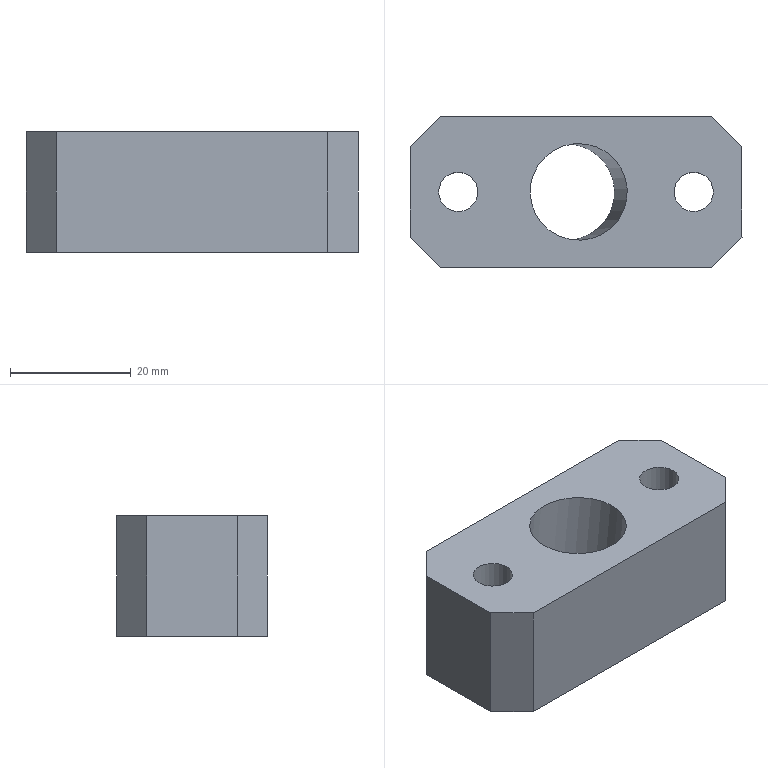Part | STEP file | P011002L001-002 | 1 solid | 17 faces | box 55 x 25 x 20 mm | volume 20325 mm3 | plane 12 | cylinder 5 | commonest cylinder face diameters 6.5 x2 11 x2 16 x1
STEP:
#1=CARTESIAN_POINT('',(0.,0.,0.));
#2=DIRECTION('',(0.,0.,1.));
#3=DIRECTION('',(1.,0.,0.));
#4=AXIS2_PLACEMENT_3D('',#1,#2,#3);
#5=CARTESIAN_POINT('',(-31.537,68.96,-131.));
#6=VERTEX_POINT('',#5);
#7=CARTESIAN_POINT('',(-34.787,68.96,-131.));
#8=DIRECTION('',(0.,0.,-1.));
#9=DIRECTION('',(1.,0.,0.));
#10=AXIS2_PLACEMENT_3D('',#7,#8,#9);
#11=CIRCLE('',#10,3.25);
#12=CARTESIAN_POINT('',(-76.791,76.46,-131.));
#13=DIRECTION('',(0.,0.,-1.));
#14=DIRECTION('',(-1.,0.,0.));
#15=AXIS2_PLACEMENT_3D('',#12,#13,#14);
#16=PLANE('',#15);
#17=CARTESIAN_POINT('',(-42.004,-7.5));
#18=DIRECTION('',(-1.,0.));
#19=AXIS2_PLACEMENT_2D('',#17,#18);
#20=CIRCLE('',#19,3.25);
#21=(GEOMETRIC_REPRESENTATION_CONTEXT(2)PARAMETRIC_REPRESENTATION_CONTEXT()REPRESENTATION_CONTEXT('',''));
#22=DEFINITIONAL_REPRESENTATION('',(#20),#21);
#23=PCURVE('',#16,#22);
#24=CARTESIAN_POINT('',(-34.787,68.96,-113.));
#25=DIRECTION('',(0.,0.,-1.));
#26=DIRECTION('',(1.,0.,0.));
#27=AXIS2_PLACEMENT_3D('',#24,#25,#26);
#28=CYLINDRICAL_SURFACE('',#27,3.25);
#29=CARTESIAN_POINT('',(0.,18.));
#30=DIRECTION('',(1.,0.));
#31=VECTOR('',#30,1.);
#32=LINE('',#29,#31);
#33=(GEOMETRIC_REPRESENTATION_CONTEXT(2)PARAMETRIC_REPRESENTATION_CONTEXT()REPRESENTATION_CONTEXT('',''));
#34=DEFINITIONAL_REPRESENTATION('',(#32),#33);
#35=PCURVE('',#28,#34);
#36=SURFACE_CURVE('',#11,(#23,#35),.PCURVE_S1.);
#37=EDGE_CURVE('',#6,#6,#36,.T.);
#38=ORIENTED_EDGE('',*,*,#37,.T.);
#39=EDGE_LOOP('',(#38));
#40=FACE_BOUND('',#39,.T.);
#41=CARTESIAN_POINT('',(-61.873,68.96,-131.));
#42=VERTEX_POINT('',#41);
#43=CARTESIAN_POINT('',(-53.828,68.96,-131.));
#44=DIRECTION('',(0.,0.,1.));
#45=DIRECTION('',(-1.,0.000000906,0.));
#46=AXIS2_PLACEMENT_3D('',#43,#44,#45);
#47=ELLIPSE('',#46,8.044,8.);
#48=CARTESIAN_POINT('',(-14.919,-7.5));
#49=CARTESIAN_POINT('',(-14.919,-21.356));
#50=CARTESIAN_POINT('',(-26.985,-14.428));
#51=CARTESIAN_POINT('',(-39.051,-7.5));
#52=CARTESIAN_POINT('',(-26.985,-0.5718));
#53=CARTESIAN_POINT('',(-14.919,6.356));
#54=CARTESIAN_POINT('',(-14.919,-7.5));
#55=(BOUNDED_CURVE()B_SPLINE_CURVE(2,(#48,#49,#50,#51,#52,#53,#54),.UNSPECIFIED.,.T.,.F.)B_SPLINE_CURVE_WITH_KNOTS((1,2,2,2,2,1),(-2.094,0.,2.094,4.189,6.283,8.378),.UNSPECIFIED.)CURVE()GEOMETRIC_REPRESENTATION_ITEM()RATIONAL_B_SPLINE_CURVE((1.,0.5,1.,0.5,1.,0.5,1.))REPRESENTATION_ITEM(''));
#56=(GEOMETRIC_REPRESENTATION_CONTEXT(2)PARAMETRIC_REPRESENTATION_CONTEXT()REPRESENTATION_CONTEXT('',''));
#57=DEFINITIONAL_REPRESENTATION('',(#55),#56);
#58=PCURVE('',#16,#57);
#59=CARTESIAN_POINT('',(-49.389,68.96,-88.759));
#60=DIRECTION('',(-0.1045,0.000000095,-0.9945));
#61=DIRECTION('',(0.9945,0.,-0.1045));
#62=AXIS2_PLACEMENT_3D('',#59,#60,#61);
#63=CYLINDRICAL_SURFACE('',#62,8.);
#64=CARTESIAN_POINT('',(9.425,43.315));
#65=CARTESIAN_POINT('',(9.33,43.315));
#66=CARTESIAN_POINT('',(9.139,43.292));
#67=CARTESIAN_POINT('',(8.854,43.191));
#68=CARTESIAN_POINT('',(8.568,43.032));
#69=CARTESIAN_POINT('',(8.282,42.828));
#70=CARTESIAN_POINT('',(7.997,42.595));
#71=CARTESIAN_POINT('',(7.711,42.353));
#72=CARTESIAN_POINT('',(7.426,42.12));
#73=CARTESIAN_POINT('',(7.14,41.916));
#74=CARTESIAN_POINT('',(6.854,41.757));
#75=CARTESIAN_POINT('',(6.569,41.656));
#76=CARTESIAN_POINT('',(6.283,41.622));
#77=CARTESIAN_POINT('',(5.998,41.656));
#78=CARTESIAN_POINT('',(5.712,41.757));
#79=CARTESIAN_POINT('',(5.426,41.916));
#80=CARTESIAN_POINT('',(5.141,42.12));
#81=CARTESIAN_POINT('',(4.855,42.353));
#82=CARTESIAN_POINT('',(4.57,42.595));
#83=CARTESIAN_POINT('',(4.284,42.828));
#84=CARTESIAN_POINT('',(3.998,43.032));
#85=CARTESIAN_POINT('',(3.713,43.191));
#86=CARTESIAN_POINT('',(3.427,43.292));
#87=CARTESIAN_POINT('',(3.237,43.315));
#88=CARTESIAN_POINT('',(3.142,43.315));
#89=B_SPLINE_CURVE_WITH_KNOTS('',3,(#64,#65,#66,#67,#68,#69,#70,#71,#72,#73,#74,#75,#76,#77,#78,#79,#80,#81,#82,#83,#84,#85,#86,#87,#88),.UNSPECIFIED.,.F.,.F.,(4,1,1,1,1,1,1,1,1,1,1,1,1,1,1,1,1,1,1,1,1,1,4),(0.,0.2856,0.5712,0.8568,1.142,1.428,1.714,1.999,2.285,2.57,2.856,3.142,3.427,3.713,3.998,4.284,4.57,4.855,5.141,5.426,5.712,5.998,6.283),.QUASI_UNIFORM_KNOTS.);
#90=(GEOMETRIC_REPRESENTATION_CONTEXT(2)PARAMETRIC_REPRESENTATION_CONTEXT()REPRESENTATION_CONTEXT('',''));
#91=DEFINITIONAL_REPRESENTATION('',(#89),#90);
#92=PCURVE('',#63,#91);
#93=SURFACE_CURVE('',#47,(#58,#92),.PCURVE_S1.);
#94=EDGE_CURVE('',#42,#42,#93,.T.);
#95=ORIENTED_EDGE('',*,*,#94,.F.);
#96=EDGE_LOOP('',(#95));
#97=FACE_BOUND('',#96,.T.);
#98=CARTESIAN_POINT('',(-76.787,81.46,-131.));
#99=VERTEX_POINT('',#98);
#100=CARTESIAN_POINT('',(-31.787,81.46,-131.));
#101=VERTEX_POINT('',#100);
#102=CARTESIAN_POINT('',(-76.791,81.46,-131.));
#103=DIRECTION('',(1.,0.,0.));
#104=VECTOR('',#103,1.);
#105=LINE('',#102,#104);
#106=CARTESIAN_POINT('',(0.,5.));
#107=DIRECTION('',(-1.,0.));
#108=VECTOR('',#107,1.);
#109=LINE('',#106,#108);
#110=(GEOMETRIC_REPRESENTATION_CONTEXT(2)PARAMETRIC_REPRESENTATION_CONTEXT()REPRESENTATION_CONTEXT('',''));
#111=DEFINITIONAL_REPRESENTATION('',(#109),#110);
#112=PCURVE('',#16,#111);
#113=CARTESIAN_POINT('',(-179.787,81.46,-246.));
#114=DIRECTION('',(0.,-1.,0.));
#115=DIRECTION('',(1.,0.,0.));
#116=AXIS2_PLACEMENT_3D('',#113,#114,#115);
#117=PLANE('',#116);
#118=CARTESIAN_POINT('',(102.996,115.));
#119=DIRECTION('',(1.,0.));
#120=VECTOR('',#119,1.);
#121=LINE('',#118,#120);
#122=(GEOMETRIC_REPRESENTATION_CONTEXT(2)PARAMETRIC_REPRESENTATION_CONTEXT()REPRESENTATION_CONTEXT('',''));
#123=DEFINITIONAL_REPRESENTATION('',(#121),#122);
#124=PCURVE('',#117,#123);
#125=SURFACE_CURVE('',#105,(#112,#124),.PCURVE_S1.);
#126=EDGE_CURVE('',#99,#101,#125,.T.);
#127=ORIENTED_EDGE('',*,*,#126,.F.);
#128=CARTESIAN_POINT('',(-81.787,76.46,-131.));
#129=VERTEX_POINT('',#128);
#130=CARTESIAN_POINT('',(-81.787,76.46,-131.));
#131=DIRECTION('',(-0.7071,-0.7071,0.));
#132=VECTOR('',#131,1.);
#133=LINE('',#130,#132);
#134=CARTESIAN_POINT('',(4.996,-0.00000231));
#135=DIRECTION('',(0.7071,-0.7071));
#136=VECTOR('',#135,1.);
#137=LINE('',#134,#136);
#138=(GEOMETRIC_REPRESENTATION_CONTEXT(2)PARAMETRIC_REPRESENTATION_CONTEXT()REPRESENTATION_CONTEXT('',''));
#139=DEFINITIONAL_REPRESENTATION('',(#137),#138);
#140=PCURVE('',#16,#139);
#141=CARTESIAN_POINT('',(-81.787,76.46,-246.));
#142=DIRECTION('',(0.7071,-0.7071,0.));
#143=DIRECTION('',(0.7071,0.7071,0.));
#144=AXIS2_PLACEMENT_3D('',#141,#142,#143);
#145=PLANE('',#144);
#146=CARTESIAN_POINT('',(0.,115.));
#147=DIRECTION('',(-1.,0.));
#148=VECTOR('',#147,1.);
#149=LINE('',#146,#148);
#150=(GEOMETRIC_REPRESENTATION_CONTEXT(2)PARAMETRIC_REPRESENTATION_CONTEXT()REPRESENTATION_CONTEXT('',''));
#151=DEFINITIONAL_REPRESENTATION('',(#149),#150);
#152=PCURVE('',#145,#151);
#153=SURFACE_CURVE('',#133,(#140,#152),.PCURVE_S1.);
#154=EDGE_CURVE('',#99,#129,#153,.T.);
#155=ORIENTED_EDGE('',*,*,#154,.T.);
#156=CARTESIAN_POINT('',(-81.787,61.46,-131.));
#157=VERTEX_POINT('',#156);
#158=CARTESIAN_POINT('',(-81.787,76.46,-131.));
#159=DIRECTION('',(0.,1.,0.));
#160=VECTOR('',#159,1.);
#161=LINE('',#158,#160);
#162=CARTESIAN_POINT('',(4.996,0.));
#163=DIRECTION('',(0.,1.));
#164=VECTOR('',#163,1.);
#165=LINE('',#162,#164);
#166=(GEOMETRIC_REPRESENTATION_CONTEXT(2)PARAMETRIC_REPRESENTATION_CONTEXT()REPRESENTATION_CONTEXT('',''));
#167=DEFINITIONAL_REPRESENTATION('',(#165),#166);
#168=PCURVE('',#16,#167);
#169=CARTESIAN_POINT('',(-81.787,-9.04,-246.));
#170=DIRECTION('',(1.,0.,0.));
#171=DIRECTION('',(0.,0.,1.));
#172=AXIS2_PLACEMENT_3D('',#169,#170,#171);
#173=PLANE('',#172);
#174=CARTESIAN_POINT('',(115.,-85.5));
#175=DIRECTION('',(0.,-1.));
#176=VECTOR('',#175,1.);
#177=LINE('',#174,#176);
#178=(GEOMETRIC_REPRESENTATION_CONTEXT(2)PARAMETRIC_REPRESENTATION_CONTEXT()REPRESENTATION_CONTEXT('',''));
#179=DEFINITIONAL_REPRESENTATION('',(#177),#178);
#180=PCURVE('',#173,#179);
#181=SURFACE_CURVE('',#161,(#168,#180),.PCURVE_S1.);
#182=EDGE_CURVE('',#157,#129,#181,.T.);
#183=ORIENTED_EDGE('',*,*,#182,.F.);
#184=CARTESIAN_POINT('',(-76.787,56.46,-131.));
#185=VERTEX_POINT('',#184);
#186=CARTESIAN_POINT('',(-76.787,56.46,-131.));
#187=DIRECTION('',(0.7071,-0.7071,0.));
#188=VECTOR('',#187,1.);
#189=LINE('',#186,#188);
#190=CARTESIAN_POINT('',(-0.004358,-20.));
#191=DIRECTION('',(-0.7071,-0.7071));
#192=VECTOR('',#191,1.);
#193=LINE('',#190,#192);
#194=(GEOMETRIC_REPRESENTATION_CONTEXT(2)PARAMETRIC_REPRESENTATION_CONTEXT()REPRESENTATION_CONTEXT('',''));
#195=DEFINITIONAL_REPRESENTATION('',(#193),#194);
#196=PCURVE('',#16,#195);
#197=CARTESIAN_POINT('',(-76.787,56.46,-131.));
#198=DIRECTION('',(-0.7071,-0.7071,0.));
#199=DIRECTION('',(0.7071,-0.7071,0.));
#200=AXIS2_PLACEMENT_3D('',#197,#198,#199);
#201=PLANE('',#200);
#202=CARTESIAN_POINT('',(0.,0.));
#203=DIRECTION('',(1.,0.));
#204=VECTOR('',#203,1.);
#205=LINE('',#202,#204);
#206=(GEOMETRIC_REPRESENTATION_CONTEXT(2)PARAMETRIC_REPRESENTATION_CONTEXT()REPRESENTATION_CONTEXT('',''));
#207=DEFINITIONAL_REPRESENTATION('',(#205),#206);
#208=PCURVE('',#201,#207);
#209=SURFACE_CURVE('',#189,(#196,#208),.PCURVE_S1.);
#210=EDGE_CURVE('',#157,#185,#209,.T.);
#211=ORIENTED_EDGE('',*,*,#210,.T.);
#212=CARTESIAN_POINT('',(-31.787,56.46,-131.));
#213=VERTEX_POINT('',#212);
#214=CARTESIAN_POINT('',(-31.791,56.46,-131.));
#215=DIRECTION('',(-1.,0.,0.));
#216=VECTOR('',#215,1.);
#217=LINE('',#214,#216);
#218=CARTESIAN_POINT('',(-45.,-20.));
#219=DIRECTION('',(1.,0.));
#220=VECTOR('',#219,1.);
#221=LINE('',#218,#220);
#222=(GEOMETRIC_REPRESENTATION_CONTEXT(2)PARAMETRIC_REPRESENTATION_CONTEXT()REPRESENTATION_CONTEXT('',''));
#223=DEFINITIONAL_REPRESENTATION('',(#221),#222);
#224=PCURVE('',#16,#223);
#225=CARTESIAN_POINT('',(-31.791,56.46,-131.));
#226=DIRECTION('',(0.,-1.,0.));
#227=DIRECTION('',(0.,0.,-1.));
#228=AXIS2_PLACEMENT_3D('',#225,#226,#227);
#229=PLANE('',#228);
#230=CARTESIAN_POINT('',(0.,0.));
#231=DIRECTION('',(0.,-1.));
#232=VECTOR('',#231,1.);
#233=LINE('',#230,#232);
#234=(GEOMETRIC_REPRESENTATION_CONTEXT(2)PARAMETRIC_REPRESENTATION_CONTEXT()REPRESENTATION_CONTEXT('',''));
#235=DEFINITIONAL_REPRESENTATION('',(#233),#234);
#236=PCURVE('',#229,#235);
#237=SURFACE_CURVE('',#217,(#224,#236),.PCURVE_S1.);
#238=EDGE_CURVE('',#213,#185,#237,.T.);
#239=ORIENTED_EDGE('',*,*,#238,.F.);
#240=CARTESIAN_POINT('',(-26.787,61.46,-131.));
#241=VERTEX_POINT('',#240);
#242=CARTESIAN_POINT('',(-26.787,61.46,-131.));
#243=DIRECTION('',(0.7071,0.7071,0.));
#244=VECTOR('',#243,1.);
#245=LINE('',#242,#244);
#246=CARTESIAN_POINT('',(-50.004,-15.));
#247=DIRECTION('',(-0.7071,0.7071));
#248=VECTOR('',#247,1.);
#249=LINE('',#246,#248);
#250=(GEOMETRIC_REPRESENTATION_CONTEXT(2)PARAMETRIC_REPRESENTATION_CONTEXT()REPRESENTATION_CONTEXT('',''));
#251=DEFINITIONAL_REPRESENTATION('',(#249),#250);
#252=PCURVE('',#16,#251);
#253=CARTESIAN_POINT('',(-26.787,61.46,-131.));
#254=DIRECTION('',(-0.7071,0.7071,0.));
#255=DIRECTION('',(-0.7071,-0.7071,0.));
#256=AXIS2_PLACEMENT_3D('',#253,#254,#255);
#257=PLANE('',#256);
#258=CARTESIAN_POINT('',(0.,0.));
#259=DIRECTION('',(-1.,0.));
#260=VECTOR('',#259,1.);
#261=LINE('',#258,#260);
#262=(GEOMETRIC_REPRESENTATION_CONTEXT(2)PARAMETRIC_REPRESENTATION_CONTEXT()REPRESENTATION_CONTEXT('',''));
#263=DEFINITIONAL_REPRESENTATION('',(#261),#262);
#264=PCURVE('',#257,#263);
#265=SURFACE_CURVE('',#245,(#252,#264),.PCURVE_S1.);
#266=EDGE_CURVE('',#213,#241,#265,.T.);
#267=ORIENTED_EDGE('',*,*,#266,.T.);
#268=CARTESIAN_POINT('',(-26.787,76.46,-131.));
#269=VERTEX_POINT('',#268);
#270=CARTESIAN_POINT('',(-26.787,76.46,-131.));
#271=DIRECTION('',(0.,-1.,0.));
#272=VECTOR('',#271,1.);
#273=LINE('',#270,#272);
#274=CARTESIAN_POINT('',(-50.004,0.));
#275=DIRECTION('',(0.,-1.));
#276=VECTOR('',#275,1.);
#277=LINE('',#274,#276);
#278=(GEOMETRIC_REPRESENTATION_CONTEXT(2)PARAMETRIC_REPRESENTATION_CONTEXT()REPRESENTATION_CONTEXT('',''));
#279=DEFINITIONAL_REPRESENTATION('',(#277),#278);
#280=PCURVE('',#16,#279);
#281=CARTESIAN_POINT('',(-26.787,76.46,-131.));
#282=DIRECTION('',(1.,0.,0.));
#283=DIRECTION('',(0.,1.,0.));
#284=AXIS2_PLACEMENT_3D('',#281,#282,#283);
#285=PLANE('',#284);
#286=CARTESIAN_POINT('',(0.,0.));
#287=DIRECTION('',(-1.,0.));
#288=VECTOR('',#287,1.);
#289=LINE('',#286,#288);
#290=(GEOMETRIC_REPRESENTATION_CONTEXT(2)PARAMETRIC_REPRESENTATION_CONTEXT()REPRESENTATION_CONTEXT('',''));
#291=DEFINITIONAL_REPRESENTATION('',(#289),#290);
#292=PCURVE('',#285,#291);
#293=SURFACE_CURVE('',#273,(#280,#292),.PCURVE_S1.);
#294=EDGE_CURVE('',#269,#241,#293,.T.);
#295=ORIENTED_EDGE('',*,*,#294,.F.);
#296=CARTESIAN_POINT('',(-31.787,81.46,-131.));
#297=DIRECTION('',(-0.7071,0.7071,0.));
#298=VECTOR('',#297,1.);
#299=LINE('',#296,#298);
#300=CARTESIAN_POINT('',(-45.004,5.));
#301=DIRECTION('',(0.7071,0.7071));
#302=VECTOR('',#301,1.);
#303=LINE('',#300,#302);
#304=(GEOMETRIC_REPRESENTATION_CONTEXT(2)PARAMETRIC_REPRESENTATION_CONTEXT()REPRESENTATION_CONTEXT('',''));
#305=DEFINITIONAL_REPRESENTATION('',(#303),#304);
#306=PCURVE('',#16,#305);
#307=CARTESIAN_POINT('',(-31.787,81.46,-246.));
#308=DIRECTION('',(0.7071,0.7071,0.));
#309=DIRECTION('',(-0.7071,0.7071,0.));
#310=AXIS2_PLACEMENT_3D('',#307,#308,#309);
#311=PLANE('',#310);
#312=CARTESIAN_POINT('',(0.,115.));
#313=DIRECTION('',(1.,0.));
#314=VECTOR('',#313,1.);
#315=LINE('',#312,#314);
#316=(GEOMETRIC_REPRESENTATION_CONTEXT(2)PARAMETRIC_REPRESENTATION_CONTEXT()REPRESENTATION_CONTEXT('',''));
#317=DEFINITIONAL_REPRESENTATION('',(#315),#316);
#318=PCURVE('',#311,#317);
#319=SURFACE_CURVE('',#299,(#306,#318),.PCURVE_S1.);
#320=EDGE_CURVE('',#269,#101,#319,.T.);
#321=ORIENTED_EDGE('',*,*,#320,.T.);
#322=EDGE_LOOP('',(#127,#155,#183,#211,#239,#267,#295,#321));
#323=FACE_BOUND('',#322,.T.);
#324=CARTESIAN_POINT('',(-70.537,68.96,-131.));
#325=VERTEX_POINT('',#324);
#326=CARTESIAN_POINT('',(-73.787,68.96,-131.));
#327=DIRECTION('',(0.,0.,-1.));
#328=DIRECTION('',(1.,0.,0.));
#329=AXIS2_PLACEMENT_3D('',#326,#327,#328);
#330=CIRCLE('',#329,3.25);
#331=CARTESIAN_POINT('',(-3.004,-7.5));
#332=DIRECTION('',(-1.,0.));
#333=AXIS2_PLACEMENT_2D('',#331,#332);
#334=CIRCLE('',#333,3.25);
#335=(GEOMETRIC_REPRESENTATION_CONTEXT(2)PARAMETRIC_REPRESENTATION_CONTEXT()REPRESENTATION_CONTEXT('',''));
#336=DEFINITIONAL_REPRESENTATION('',(#334),#335);
#337=PCURVE('',#16,#336);
#338=CARTESIAN_POINT('',(-73.787,68.96,-113.));
#339=DIRECTION('',(0.,0.,-1.));
#340=DIRECTION('',(-1.,0.,0.));
#341=AXIS2_PLACEMENT_3D('',#338,#339,#340);
#342=CYLINDRICAL_SURFACE('',#341,3.25);
#343=CARTESIAN_POINT('',(3.142,18.));
#344=DIRECTION('',(1.,0.));
#345=VECTOR('',#344,1.);
#346=LINE('',#343,#345);
#347=(GEOMETRIC_REPRESENTATION_CONTEXT(2)PARAMETRIC_REPRESENTATION_CONTEXT()REPRESENTATION_CONTEXT('',''));
#348=DEFINITIONAL_REPRESENTATION('',(#346),#347);
#349=PCURVE('',#342,#348);
#350=SURFACE_CURVE('',#330,(#337,#349),.PCURVE_S1.);
#351=EDGE_CURVE('',#325,#325,#350,.T.);
#352=ORIENTED_EDGE('',*,*,#351,.T.);
#353=EDGE_LOOP('',(#352));
#354=FACE_BOUND('',#353,.T.);
#355=ADVANCED_FACE('',(#40,#97,#323,#354),#16,.F.);
#356=CARTESIAN_POINT('',(-68.287,68.96,-151.));
#357=VERTEX_POINT('',#356);
#358=CARTESIAN_POINT('',(-73.787,68.96,-151.));
#359=DIRECTION('',(0.,0.,1.));
#360=DIRECTION('',(1.,0.,0.));
#361=AXIS2_PLACEMENT_3D('',#358,#359,#360);
#362=CIRCLE('',#361,5.5);
#363=CARTESIAN_POINT('',(-76.791,76.46,-151.));
#364=DIRECTION('',(0.,0.,-1.));
#365=DIRECTION('',(-1.,0.,0.));
#366=AXIS2_PLACEMENT_3D('',#363,#364,#365);
#367=PLANE('',#366);
#368=CARTESIAN_POINT('',(-8.504,-7.5));
#369=CARTESIAN_POINT('',(-8.504,2.026));
#370=CARTESIAN_POINT('',(-0.2544,-2.737));
#371=CARTESIAN_POINT('',(7.996,-7.5));
#372=CARTESIAN_POINT('',(-0.2544,-12.263));
#373=CARTESIAN_POINT('',(-8.504,-17.026));
#374=CARTESIAN_POINT('',(-8.504,-7.5));
#375=(BOUNDED_CURVE()B_SPLINE_CURVE(2,(#368,#369,#370,#371,#372,#373,#374),.UNSPECIFIED.,.T.,.F.)B_SPLINE_CURVE_WITH_KNOTS((1,2,2,2,2,1),(-2.094,0.,2.094,4.189,6.283,8.378),.UNSPECIFIED.)CURVE()GEOMETRIC_REPRESENTATION_ITEM()RATIONAL_B_SPLINE_CURVE((1.,0.5,1.,0.5,1.,0.5,1.))REPRESENTATION_ITEM(''));
#376=(GEOMETRIC_REPRESENTATION_CONTEXT(2)PARAMETRIC_REPRESENTATION_CONTEXT()REPRESENTATION_CONTEXT('',''));
#377=DEFINITIONAL_REPRESENTATION('',(#375),#376);
#378=PCURVE('',#367,#377);
#379=CARTESIAN_POINT('',(-73.787,68.96,-113.));
#380=DIRECTION('',(0.,0.,-1.));
#381=DIRECTION('',(-1.,0.,0.));
#382=AXIS2_PLACEMENT_3D('',#379,#380,#381);
#383=CYLINDRICAL_SURFACE('',#382,5.5);
#384=CARTESIAN_POINT('',(9.425,38.));
#385=DIRECTION('',(-1.,0.));
#386=VECTOR('',#385,1.);
#387=LINE('',#384,#386);
#388=(GEOMETRIC_REPRESENTATION_CONTEXT(2)PARAMETRIC_REPRESENTATION_CONTEXT()REPRESENTATION_CONTEXT('',''));
#389=DEFINITIONAL_REPRESENTATION('',(#387),#388);
#390=PCURVE('',#383,#389);
#391=SURFACE_CURVE('',#362,(#378,#390),.PCURVE_S1.);
#392=EDGE_CURVE('',#357,#357,#391,.T.);
#393=ORIENTED_EDGE('',*,*,#392,.T.);
#394=EDGE_LOOP('',(#393));
#395=FACE_BOUND('',#394,.T.);
#396=CARTESIAN_POINT('',(-81.787,61.46,-151.));
#397=VERTEX_POINT('',#396);
#398=CARTESIAN_POINT('',(-81.787,76.46,-151.));
#399=VERTEX_POINT('',#398);
#400=CARTESIAN_POINT('',(-81.787,76.46,-151.));
#401=DIRECTION('',(0.,1.,0.));
#402=VECTOR('',#401,1.);
#403=LINE('',#400,#402);
#404=CARTESIAN_POINT('',(4.996,0.));
#405=DIRECTION('',(0.,1.));
#406=VECTOR('',#405,1.);
#407=LINE('',#404,#406);
#408=(GEOMETRIC_REPRESENTATION_CONTEXT(2)PARAMETRIC_REPRESENTATION_CONTEXT()REPRESENTATION_CONTEXT('',''));
#409=DEFINITIONAL_REPRESENTATION('',(#407),#408);
#410=PCURVE('',#367,#409);
#411=CARTESIAN_POINT('',(95.,-85.5));
#412=DIRECTION('',(0.,-1.));
#413=VECTOR('',#412,1.);
#414=LINE('',#411,#413);
#415=(GEOMETRIC_REPRESENTATION_CONTEXT(2)PARAMETRIC_REPRESENTATION_CONTEXT()REPRESENTATION_CONTEXT('',''));
#416=DEFINITIONAL_REPRESENTATION('',(#414),#415);
#417=PCURVE('',#173,#416);
#418=SURFACE_CURVE('',#403,(#410,#417),.PCURVE_S1.);
#419=EDGE_CURVE('',#397,#399,#418,.T.);
#420=ORIENTED_EDGE('',*,*,#419,.T.);
#421=CARTESIAN_POINT('',(-76.787,81.46,-151.));
#422=VERTEX_POINT('',#421);
#423=CARTESIAN_POINT('',(-79.289,78.958,-151.));
#424=DIRECTION('',(0.7071,0.7071,0.));
#425=VECTOR('',#424,1.);
#426=LINE('',#423,#425);
#427=CARTESIAN_POINT('',(2.498,2.498));
#428=DIRECTION('',(-0.7071,0.7071));
#429=VECTOR('',#428,1.);
#430=LINE('',#427,#429);
#431=(GEOMETRIC_REPRESENTATION_CONTEXT(2)PARAMETRIC_REPRESENTATION_CONTEXT()REPRESENTATION_CONTEXT('',''));
#432=DEFINITIONAL_REPRESENTATION('',(#430),#431);
#433=PCURVE('',#367,#432);
#434=CARTESIAN_POINT('',(3.532,95.));
#435=DIRECTION('',(1.,0.));
#436=VECTOR('',#435,1.);
#437=LINE('',#434,#436);
#438=(GEOMETRIC_REPRESENTATION_CONTEXT(2)PARAMETRIC_REPRESENTATION_CONTEXT()REPRESENTATION_CONTEXT('',''));
#439=DEFINITIONAL_REPRESENTATION('',(#437),#438);
#440=PCURVE('',#145,#439);
#441=SURFACE_CURVE('',#426,(#433,#440),.PCURVE_S1.);
#442=EDGE_CURVE('',#399,#422,#441,.T.);
#443=ORIENTED_EDGE('',*,*,#442,.T.);
#444=CARTESIAN_POINT('',(-31.787,81.46,-151.));
#445=VERTEX_POINT('',#444);
#446=CARTESIAN_POINT('',(-76.791,81.46,-151.));
#447=DIRECTION('',(1.,0.,0.));
#448=VECTOR('',#447,1.);
#449=LINE('',#446,#448);
#450=CARTESIAN_POINT('',(0.,5.));
#451=DIRECTION('',(-1.,0.));
#452=VECTOR('',#451,1.);
#453=LINE('',#450,#452);
#454=(GEOMETRIC_REPRESENTATION_CONTEXT(2)PARAMETRIC_REPRESENTATION_CONTEXT()REPRESENTATION_CONTEXT('',''));
#455=DEFINITIONAL_REPRESENTATION('',(#453),#454);
#456=PCURVE('',#367,#455);
#457=CARTESIAN_POINT('',(102.996,95.));
#458=DIRECTION('',(1.,0.));
#459=VECTOR('',#458,1.);
#460=LINE('',#457,#459);
#461=(GEOMETRIC_REPRESENTATION_CONTEXT(2)PARAMETRIC_REPRESENTATION_CONTEXT()REPRESENTATION_CONTEXT('',''));
#462=DEFINITIONAL_REPRESENTATION('',(#460),#461);
#463=PCURVE('',#117,#462);
#464=SURFACE_CURVE('',#449,(#456,#463),.PCURVE_S1.);
#465=EDGE_CURVE('',#422,#445,#464,.T.);
#466=ORIENTED_EDGE('',*,*,#465,.T.);
#467=CARTESIAN_POINT('',(-26.787,76.46,-151.));
#468=VERTEX_POINT('',#467);
#469=CARTESIAN_POINT('',(-51.789,101.462,-151.));
#470=DIRECTION('',(0.7071,-0.7071,0.));
#471=VECTOR('',#470,1.);
#472=LINE('',#469,#471);
#473=CARTESIAN_POINT('',(-25.002,25.002));
#474=DIRECTION('',(-0.7071,-0.7071));
#475=VECTOR('',#474,1.);
#476=LINE('',#473,#475);
#477=(GEOMETRIC_REPRESENTATION_CONTEXT(2)PARAMETRIC_REPRESENTATION_CONTEXT()REPRESENTATION_CONTEXT('',''));
#478=DEFINITIONAL_REPRESENTATION('',(#476),#477);
#479=PCURVE('',#367,#478);
#480=CARTESIAN_POINT('',(28.287,95.));
#481=DIRECTION('',(-1.,0.));
#482=VECTOR('',#481,1.);
#483=LINE('',#480,#482);
#484=(GEOMETRIC_REPRESENTATION_CONTEXT(2)PARAMETRIC_REPRESENTATION_CONTEXT()REPRESENTATION_CONTEXT('',''));
#485=DEFINITIONAL_REPRESENTATION('',(#483),#484);
#486=PCURVE('',#311,#485);
#487=SURFACE_CURVE('',#472,(#479,#486),.PCURVE_S1.);
#488=EDGE_CURVE('',#445,#468,#487,.T.);
#489=ORIENTED_EDGE('',*,*,#488,.T.);
#490=CARTESIAN_POINT('',(-26.787,61.46,-151.));
#491=VERTEX_POINT('',#490);
#492=CARTESIAN_POINT('',(-26.787,76.46,-151.));
#493=DIRECTION('',(0.,-1.,0.));
#494=VECTOR('',#493,1.);
#495=LINE('',#492,#494);
#496=CARTESIAN_POINT('',(-50.004,0.));
#497=DIRECTION('',(0.,-1.));
#498=VECTOR('',#497,1.);
#499=LINE('',#496,#498);
#500=(GEOMETRIC_REPRESENTATION_CONTEXT(2)PARAMETRIC_REPRESENTATION_CONTEXT()REPRESENTATION_CONTEXT('',''));
#501=DEFINITIONAL_REPRESENTATION('',(#499),#500);
#502=PCURVE('',#367,#501);
#503=CARTESIAN_POINT('',(0.,-20.));
#504=DIRECTION('',(-1.,0.));
#505=VECTOR('',#504,1.);
#506=LINE('',#503,#505);
#507=(GEOMETRIC_REPRESENTATION_CONTEXT(2)PARAMETRIC_REPRESENTATION_CONTEXT()REPRESENTATION_CONTEXT('',''));
#508=DEFINITIONAL_REPRESENTATION('',(#506),#507);
#509=PCURVE('',#285,#508);
#510=SURFACE_CURVE('',#495,(#502,#509),.PCURVE_S1.);
#511=EDGE_CURVE('',#468,#491,#510,.T.);
#512=ORIENTED_EDGE('',*,*,#511,.T.);
#513=CARTESIAN_POINT('',(-31.787,56.46,-151.));
#514=VERTEX_POINT('',#513);
#515=CARTESIAN_POINT('',(-44.289,43.958,-151.));
#516=DIRECTION('',(-0.7071,-0.7071,0.));
#517=VECTOR('',#516,1.);
#518=LINE('',#515,#517);
#519=CARTESIAN_POINT('',(-32.502,-32.502));
#520=DIRECTION('',(0.7071,-0.7071));
#521=VECTOR('',#520,1.);
#522=LINE('',#519,#521);
#523=(GEOMETRIC_REPRESENTATION_CONTEXT(2)PARAMETRIC_REPRESENTATION_CONTEXT()REPRESENTATION_CONTEXT('',''));
#524=DEFINITIONAL_REPRESENTATION('',(#522),#523);
#525=PCURVE('',#367,#524);
#526=CARTESIAN_POINT('',(24.752,-20.));
#527=DIRECTION('',(1.,0.));
#528=VECTOR('',#527,1.);
#529=LINE('',#526,#528);
#530=(GEOMETRIC_REPRESENTATION_CONTEXT(2)PARAMETRIC_REPRESENTATION_CONTEXT()REPRESENTATION_CONTEXT('',''));
#531=DEFINITIONAL_REPRESENTATION('',(#529),#530);
#532=PCURVE('',#257,#531);
#533=SURFACE_CURVE('',#518,(#525,#532),.PCURVE_S1.);
#534=EDGE_CURVE('',#491,#514,#533,.T.);
#535=ORIENTED_EDGE('',*,*,#534,.T.);
#536=CARTESIAN_POINT('',(-76.787,56.46,-151.));
#537=VERTEX_POINT('',#536);
#538=CARTESIAN_POINT('',(-31.791,56.46,-151.));
#539=DIRECTION('',(-1.,0.,0.));
#540=VECTOR('',#539,1.);
#541=LINE('',#538,#540);
#542=CARTESIAN_POINT('',(-45.,-20.));
#543=DIRECTION('',(1.,0.));
#544=VECTOR('',#543,1.);
#545=LINE('',#542,#544);
#546=(GEOMETRIC_REPRESENTATION_CONTEXT(2)PARAMETRIC_REPRESENTATION_CONTEXT()REPRESENTATION_CONTEXT('',''));
#547=DEFINITIONAL_REPRESENTATION('',(#545),#546);
#548=PCURVE('',#367,#547);
#549=CARTESIAN_POINT('',(20.,0.));
#550=DIRECTION('',(0.,-1.));
#551=VECTOR('',#550,1.);
#552=LINE('',#549,#551);
#553=(GEOMETRIC_REPRESENTATION_CONTEXT(2)PARAMETRIC_REPRESENTATION_CONTEXT()REPRESENTATION_CONTEXT('',''));
#554=DEFINITIONAL_REPRESENTATION('',(#552),#553);
#555=PCURVE('',#229,#554);
#556=SURFACE_CURVE('',#541,(#548,#555),.PCURVE_S1.);
#557=EDGE_CURVE('',#514,#537,#556,.T.);
#558=ORIENTED_EDGE('',*,*,#557,.T.);
#559=CARTESIAN_POINT('',(-86.789,66.462,-151.));
#560=DIRECTION('',(-0.7071,0.7071,0.));
#561=VECTOR('',#560,1.);
#562=LINE('',#559,#561);
#563=CARTESIAN_POINT('',(9.998,-9.998));
#564=DIRECTION('',(0.7071,0.7071));
#565=VECTOR('',#564,1.);
#566=LINE('',#563,#565);
#567=(GEOMETRIC_REPRESENTATION_CONTEXT(2)PARAMETRIC_REPRESENTATION_CONTEXT()REPRESENTATION_CONTEXT('',''));
#568=DEFINITIONAL_REPRESENTATION('',(#566),#567);
#569=PCURVE('',#367,#568);
#570=CARTESIAN_POINT('',(-14.145,-20.));
#571=DIRECTION('',(-1.,0.));
#572=VECTOR('',#571,1.);
#573=LINE('',#570,#572);
#574=(GEOMETRIC_REPRESENTATION_CONTEXT(2)PARAMETRIC_REPRESENTATION_CONTEXT()REPRESENTATION_CONTEXT('',''));
#575=DEFINITIONAL_REPRESENTATION('',(#573),#574);
#576=PCURVE('',#201,#575);
#577=SURFACE_CURVE('',#562,(#569,#576),.PCURVE_S1.);
#578=EDGE_CURVE('',#537,#397,#577,.T.);
#579=ORIENTED_EDGE('',*,*,#578,.T.);
#580=EDGE_LOOP('',(#420,#443,#466,#489,#512,#535,#558,#579));
#581=FACE_BOUND('',#580,.T.);
#582=CARTESIAN_POINT('',(-63.975,68.96,-151.));
#583=VERTEX_POINT('',#582);
#584=CARTESIAN_POINT('',(-55.931,68.96,-151.));
#585=DIRECTION('',(0.,0.,1.));
#586=DIRECTION('',(-1.,0.000000906,0.));
#587=AXIS2_PLACEMENT_3D('',#584,#585,#586);
#588=ELLIPSE('',#587,8.044,8.);
#589=CARTESIAN_POINT('',(-12.816,-7.5));
#590=CARTESIAN_POINT('',(-12.816,-21.356));
#591=CARTESIAN_POINT('',(-24.883,-14.428));
#592=CARTESIAN_POINT('',(-36.949,-7.5));
#593=CARTESIAN_POINT('',(-24.883,-0.5718));
#594=CARTESIAN_POINT('',(-12.816,6.356));
#595=CARTESIAN_POINT('',(-12.816,-7.5));
#596=(BOUNDED_CURVE()B_SPLINE_CURVE(2,(#589,#590,#591,#592,#593,#594,#595),.UNSPECIFIED.,.T.,.F.)B_SPLINE_CURVE_WITH_KNOTS((1,2,2,2,2,1),(-2.094,0.,2.094,4.189,6.283,8.378),.UNSPECIFIED.)CURVE()GEOMETRIC_REPRESENTATION_ITEM()RATIONAL_B_SPLINE_CURVE((1.,0.5,1.,0.5,1.,0.5,1.))REPRESENTATION_ITEM(''));
#597=(GEOMETRIC_REPRESENTATION_CONTEXT(2)PARAMETRIC_REPRESENTATION_CONTEXT()REPRESENTATION_CONTEXT('',''));
#598=DEFINITIONAL_REPRESENTATION('',(#596),#597);
#599=PCURVE('',#367,#598);
#600=CARTESIAN_POINT('',(9.425,63.425));
#601=CARTESIAN_POINT('',(9.33,63.426));
#602=CARTESIAN_POINT('',(9.139,63.402));
#603=CARTESIAN_POINT('',(8.854,63.301));
#604=CARTESIAN_POINT('',(8.568,63.142));
#605=CARTESIAN_POINT('',(8.282,62.938));
#606=CARTESIAN_POINT('',(7.997,62.706));
#607=CARTESIAN_POINT('',(7.711,62.463));
#608=CARTESIAN_POINT('',(7.426,62.23));
#609=CARTESIAN_POINT('',(7.14,62.026));
#610=CARTESIAN_POINT('',(6.854,61.867));
#611=CARTESIAN_POINT('',(6.569,61.766));
#612=CARTESIAN_POINT('',(6.283,61.732));
#613=CARTESIAN_POINT('',(5.998,61.766));
#614=CARTESIAN_POINT('',(5.712,61.867));
#615=CARTESIAN_POINT('',(5.426,62.026));
#616=CARTESIAN_POINT('',(5.141,62.23));
#617=CARTESIAN_POINT('',(4.855,62.463));
#618=CARTESIAN_POINT('',(4.57,62.706));
#619=CARTESIAN_POINT('',(4.284,62.938));
#620=CARTESIAN_POINT('',(3.998,63.142));
#621=CARTESIAN_POINT('',(3.713,63.301));
#622=CARTESIAN_POINT('',(3.427,63.402));
#623=CARTESIAN_POINT('',(3.237,63.426));
#624=CARTESIAN_POINT('',(3.142,63.425));
#625=B_SPLINE_CURVE_WITH_KNOTS('',3,(#600,#601,#602,#603,#604,#605,#606,#607,#608,#609,#610,#611,#612,#613,#614,#615,#616,#617,#618,#619,#620,#621,#622,#623,#624),.UNSPECIFIED.,.F.,.F.,(4,1,1,1,1,1,1,1,1,1,1,1,1,1,1,1,1,1,1,1,1,1,4),(0.,0.2856,0.5712,0.8568,1.142,1.428,1.714,1.999,2.285,2.57,2.856,3.142,3.427,3.713,3.998,4.284,4.57,4.855,5.141,5.426,5.712,5.998,6.283),.QUASI_UNIFORM_KNOTS.);
#626=(GEOMETRIC_REPRESENTATION_CONTEXT(2)PARAMETRIC_REPRESENTATION_CONTEXT()REPRESENTATION_CONTEXT('',''));
#627=DEFINITIONAL_REPRESENTATION('',(#625),#626);
#628=PCURVE('',#63,#627);
#629=SURFACE_CURVE('',#588,(#599,#628),.PCURVE_S1.);
#630=EDGE_CURVE('',#583,#583,#629,.T.);
#631=ORIENTED_EDGE('',*,*,#630,.T.);
#632=EDGE_LOOP('',(#631));
#633=FACE_BOUND('',#632,.T.);
#634=CARTESIAN_POINT('',(-40.287,68.96,-151.));
#635=VERTEX_POINT('',#634);
#636=CARTESIAN_POINT('',(-34.787,68.96,-151.));
#637=DIRECTION('',(0.,0.,-1.));
#638=DIRECTION('',(-1.,0.,0.));
#639=AXIS2_PLACEMENT_3D('',#636,#637,#638);
#640=CIRCLE('',#639,5.5);
#641=CARTESIAN_POINT('',(-42.004,-7.5));
#642=DIRECTION('',(1.,0.));
#643=AXIS2_PLACEMENT_2D('',#641,#642);
#644=CIRCLE('',#643,5.5);
#645=(GEOMETRIC_REPRESENTATION_CONTEXT(2)PARAMETRIC_REPRESENTATION_CONTEXT()REPRESENTATION_CONTEXT('',''));
#646=DEFINITIONAL_REPRESENTATION('',(#644),#645);
#647=PCURVE('',#367,#646);
#648=CARTESIAN_POINT('',(-34.787,68.96,-113.));
#649=DIRECTION('',(0.,0.,-1.));
#650=DIRECTION('',(1.,0.,0.));
#651=AXIS2_PLACEMENT_3D('',#648,#649,#650);
#652=CYLINDRICAL_SURFACE('',#651,5.5);
#653=CARTESIAN_POINT('',(3.142,38.));
#654=DIRECTION('',(1.,0.));
#655=VECTOR('',#654,1.);
#656=LINE('',#653,#655);
#657=(GEOMETRIC_REPRESENTATION_CONTEXT(2)PARAMETRIC_REPRESENTATION_CONTEXT()REPRESENTATION_CONTEXT('',''));
#658=DEFINITIONAL_REPRESENTATION('',(#656),#657);
#659=PCURVE('',#652,#658);
#660=SURFACE_CURVE('',#640,(#647,#659),.PCURVE_S1.);
#661=EDGE_CURVE('',#635,#635,#660,.T.);
#662=ORIENTED_EDGE('',*,*,#661,.F.);
#663=EDGE_LOOP('',(#662));
#664=FACE_BOUND('',#663,.T.);
#665=ADVANCED_FACE('',(#395,#581,#633,#664),#367,.T.);
#666=ORIENTED_EDGE('',*,*,#465,.F.);
#667=CARTESIAN_POINT('',(-76.787,81.46,-246.));
#668=DIRECTION('',(0.,0.,1.));
#669=VECTOR('',#668,1.);
#670=LINE('',#667,#669);
#671=CARTESIAN_POINT('',(103.,0.));
#672=DIRECTION('',(0.,1.));
#673=VECTOR('',#672,1.);
#674=LINE('',#671,#673);
#675=(GEOMETRIC_REPRESENTATION_CONTEXT(2)PARAMETRIC_REPRESENTATION_CONTEXT()REPRESENTATION_CONTEXT('',''));
#676=DEFINITIONAL_REPRESENTATION('',(#674),#675);
#677=PCURVE('',#117,#676);
#678=CARTESIAN_POINT('',(7.071,0.));
#679=DIRECTION('',(0.,1.));
#680=VECTOR('',#679,1.);
#681=LINE('',#678,#680);
#682=(GEOMETRIC_REPRESENTATION_CONTEXT(2)PARAMETRIC_REPRESENTATION_CONTEXT()REPRESENTATION_CONTEXT('',''));
#683=DEFINITIONAL_REPRESENTATION('',(#681),#682);
#684=PCURVE('',#145,#683);
#685=SURFACE_CURVE('',#670,(#677,#684),.PCURVE_S1.);
#686=EDGE_CURVE('',#422,#99,#685,.T.);
#687=ORIENTED_EDGE('',*,*,#686,.T.);
#688=ORIENTED_EDGE('',*,*,#126,.T.);
#689=CARTESIAN_POINT('',(-31.787,81.46,-246.));
#690=DIRECTION('',(0.,0.,-1.));
#691=VECTOR('',#690,1.);
#692=LINE('',#689,#691);
#693=CARTESIAN_POINT('',(148.,0.));
#694=DIRECTION('',(0.,-1.));
#695=VECTOR('',#694,1.);
#696=LINE('',#693,#695);
#697=(GEOMETRIC_REPRESENTATION_CONTEXT(2)PARAMETRIC_REPRESENTATION_CONTEXT()REPRESENTATION_CONTEXT('',''));
#698=DEFINITIONAL_REPRESENTATION('',(#696),#697);
#699=PCURVE('',#117,#698);
#700=CARTESIAN_POINT('',(0.,0.));
#701=DIRECTION('',(0.,-1.));
#702=VECTOR('',#701,1.);
#703=LINE('',#700,#702);
#704=(GEOMETRIC_REPRESENTATION_CONTEXT(2)PARAMETRIC_REPRESENTATION_CONTEXT()REPRESENTATION_CONTEXT('',''));
#705=DEFINITIONAL_REPRESENTATION('',(#703),#704);
#706=PCURVE('',#311,#705);
#707=SURFACE_CURVE('',#692,(#699,#706),.PCURVE_S1.);
#708=EDGE_CURVE('',#101,#445,#707,.T.);
#709=ORIENTED_EDGE('',*,*,#708,.T.);
#710=EDGE_LOOP('',(#666,#687,#688,#709));
#711=FACE_BOUND('',#710,.T.);
#712=ADVANCED_FACE('',(#711),#117,.F.);
#713=ORIENTED_EDGE('',*,*,#511,.F.);
#714=CARTESIAN_POINT('',(-26.787,76.46,-131.));
#715=DIRECTION('',(0.,0.,1.));
#716=VECTOR('',#715,1.);
#717=LINE('',#714,#716);
#718=CARTESIAN_POINT('',(-0.000002305,0.));
#719=DIRECTION('',(0.,1.));
#720=VECTOR('',#719,1.);
#721=LINE('',#718,#720);
#722=(GEOMETRIC_REPRESENTATION_CONTEXT(2)PARAMETRIC_REPRESENTATION_CONTEXT()REPRESENTATION_CONTEXT('',''));
#723=DEFINITIONAL_REPRESENTATION('',(#721),#722);
#724=PCURVE('',#285,#723);
#725=CARTESIAN_POINT('',(-7.071,115.));
#726=DIRECTION('',(0.,1.));
#727=VECTOR('',#726,1.);
#728=LINE('',#725,#727);
#729=(GEOMETRIC_REPRESENTATION_CONTEXT(2)PARAMETRIC_REPRESENTATION_CONTEXT()REPRESENTATION_CONTEXT('',''));
#730=DEFINITIONAL_REPRESENTATION('',(#728),#729);
#731=PCURVE('',#311,#730);
#732=SURFACE_CURVE('',#717,(#724,#731),.PCURVE_S1.);
#733=EDGE_CURVE('',#468,#269,#732,.T.);
#734=ORIENTED_EDGE('',*,*,#733,.T.);
#735=ORIENTED_EDGE('',*,*,#294,.T.);
#736=CARTESIAN_POINT('',(-26.787,61.46,-131.));
#737=DIRECTION('',(0.,0.,-1.));
#738=VECTOR('',#737,1.);
#739=LINE('',#736,#738);
#740=CARTESIAN_POINT('',(-15.,0.));
#741=DIRECTION('',(0.,-1.));
#742=VECTOR('',#741,1.);
#743=LINE('',#740,#742);
#744=(GEOMETRIC_REPRESENTATION_CONTEXT(2)PARAMETRIC_REPRESENTATION_CONTEXT()REPRESENTATION_CONTEXT('',''));
#745=DEFINITIONAL_REPRESENTATION('',(#743),#744);
#746=PCURVE('',#285,#745);
#747=CARTESIAN_POINT('',(0.,0.));
#748=DIRECTION('',(0.,-1.));
#749=VECTOR('',#748,1.);
#750=LINE('',#747,#749);
#751=(GEOMETRIC_REPRESENTATION_CONTEXT(2)PARAMETRIC_REPRESENTATION_CONTEXT()REPRESENTATION_CONTEXT('',''));
#752=DEFINITIONAL_REPRESENTATION('',(#750),#751);
#753=PCURVE('',#257,#752);
#754=SURFACE_CURVE('',#739,(#746,#753),.PCURVE_S1.);
#755=EDGE_CURVE('',#241,#491,#754,.T.);
#756=ORIENTED_EDGE('',*,*,#755,.T.);
#757=EDGE_LOOP('',(#713,#734,#735,#756));
#758=FACE_BOUND('',#757,.T.);
#759=ADVANCED_FACE('',(#758),#285,.T.);
#760=ORIENTED_EDGE('',*,*,#557,.F.);
#761=CARTESIAN_POINT('',(-31.787,56.46,-131.));
#762=DIRECTION('',(0.,0.,1.));
#763=VECTOR('',#762,1.);
#764=LINE('',#761,#763);
#765=CARTESIAN_POINT('',(0.,0.004358));
#766=DIRECTION('',(-1.,0.));
#767=VECTOR('',#766,1.);
#768=LINE('',#765,#767);
#769=(GEOMETRIC_REPRESENTATION_CONTEXT(2)PARAMETRIC_REPRESENTATION_CONTEXT()REPRESENTATION_CONTEXT('',''));
#770=DEFINITIONAL_REPRESENTATION('',(#768),#769);
#771=PCURVE('',#229,#770);
#772=CARTESIAN_POINT('',(7.071,0.));
#773=DIRECTION('',(0.,1.));
#774=VECTOR('',#773,1.);
#775=LINE('',#772,#774);
#776=(GEOMETRIC_REPRESENTATION_CONTEXT(2)PARAMETRIC_REPRESENTATION_CONTEXT()REPRESENTATION_CONTEXT('',''));
#777=DEFINITIONAL_REPRESENTATION('',(#775),#776);
#778=PCURVE('',#257,#777);
#779=SURFACE_CURVE('',#764,(#771,#778),.PCURVE_S1.);
#780=EDGE_CURVE('',#514,#213,#779,.T.);
#781=ORIENTED_EDGE('',*,*,#780,.T.);
#782=ORIENTED_EDGE('',*,*,#238,.T.);
#783=CARTESIAN_POINT('',(-76.787,56.46,-131.));
#784=DIRECTION('',(0.,0.,-1.));
#785=VECTOR('',#784,1.);
#786=LINE('',#783,#785);
#787=CARTESIAN_POINT('',(0.,-44.996));
#788=DIRECTION('',(1.,0.));
#789=VECTOR('',#788,1.);
#790=LINE('',#787,#789);
#791=(GEOMETRIC_REPRESENTATION_CONTEXT(2)PARAMETRIC_REPRESENTATION_CONTEXT()REPRESENTATION_CONTEXT('',''));
#792=DEFINITIONAL_REPRESENTATION('',(#790),#791);
#793=PCURVE('',#229,#792);
#794=CARTESIAN_POINT('',(0.,0.));
#795=DIRECTION('',(0.,-1.));
#796=VECTOR('',#795,1.);
#797=LINE('',#794,#796);
#798=(GEOMETRIC_REPRESENTATION_CONTEXT(2)PARAMETRIC_REPRESENTATION_CONTEXT()REPRESENTATION_CONTEXT('',''));
#799=DEFINITIONAL_REPRESENTATION('',(#797),#798);
#800=PCURVE('',#201,#799);
#801=SURFACE_CURVE('',#786,(#793,#800),.PCURVE_S1.);
#802=EDGE_CURVE('',#185,#537,#801,.T.);
#803=ORIENTED_EDGE('',*,*,#802,.T.);
#804=EDGE_LOOP('',(#760,#781,#782,#803));
#805=FACE_BOUND('',#804,.T.);
#806=ADVANCED_FACE('',(#805),#229,.T.);
#807=ORIENTED_EDGE('',*,*,#182,.T.);
#808=CARTESIAN_POINT('',(-81.787,76.46,-246.));
#809=DIRECTION('',(0.,0.,-1.));
#810=VECTOR('',#809,1.);
#811=LINE('',#808,#810);
#812=CARTESIAN_POINT('',(0.,-85.5));
#813=DIRECTION('',(-1.,0.));
#814=VECTOR('',#813,1.);
#815=LINE('',#812,#814);
#816=(GEOMETRIC_REPRESENTATION_CONTEXT(2)PARAMETRIC_REPRESENTATION_CONTEXT()REPRESENTATION_CONTEXT('',''));
#817=DEFINITIONAL_REPRESENTATION('',(#815),#816);
#818=PCURVE('',#173,#817);
#819=CARTESIAN_POINT('',(0.,0.));
#820=DIRECTION('',(0.,-1.));
#821=VECTOR('',#820,1.);
#822=LINE('',#819,#821);
#823=(GEOMETRIC_REPRESENTATION_CONTEXT(2)PARAMETRIC_REPRESENTATION_CONTEXT()REPRESENTATION_CONTEXT('',''));
#824=DEFINITIONAL_REPRESENTATION('',(#822),#823);
#825=PCURVE('',#145,#824);
#826=SURFACE_CURVE('',#811,(#818,#825),.PCURVE_S1.);
#827=EDGE_CURVE('',#129,#399,#826,.T.);
#828=ORIENTED_EDGE('',*,*,#827,.T.);
#829=ORIENTED_EDGE('',*,*,#419,.F.);
#830=CARTESIAN_POINT('',(-81.787,61.46,-246.));
#831=DIRECTION('',(0.,0.,1.));
#832=VECTOR('',#831,1.);
#833=LINE('',#830,#832);
#834=CARTESIAN_POINT('',(0.,-70.5));
#835=DIRECTION('',(1.,0.));
#836=VECTOR('',#835,1.);
#837=LINE('',#834,#836);
#838=(GEOMETRIC_REPRESENTATION_CONTEXT(2)PARAMETRIC_REPRESENTATION_CONTEXT()REPRESENTATION_CONTEXT('',''));
#839=DEFINITIONAL_REPRESENTATION('',(#837),#838);
#840=PCURVE('',#173,#839);
#841=CARTESIAN_POINT('',(-7.071,-115.));
#842=DIRECTION('',(0.,1.));
#843=VECTOR('',#842,1.);
#844=LINE('',#841,#843);
#845=(GEOMETRIC_REPRESENTATION_CONTEXT(2)PARAMETRIC_REPRESENTATION_CONTEXT()REPRESENTATION_CONTEXT('',''));
#846=DEFINITIONAL_REPRESENTATION('',(#844),#845);
#847=PCURVE('',#201,#846);
#848=SURFACE_CURVE('',#833,(#840,#847),.PCURVE_S1.);
#849=EDGE_CURVE('',#397,#157,#848,.T.);
#850=ORIENTED_EDGE('',*,*,#849,.T.);
#851=EDGE_LOOP('',(#807,#828,#829,#850));
#852=FACE_BOUND('',#851,.T.);
#853=ADVANCED_FACE('',(#852),#173,.F.);
#854=ORIENTED_EDGE('',*,*,#154,.F.);
#855=ORIENTED_EDGE('',*,*,#686,.F.);
#856=ORIENTED_EDGE('',*,*,#442,.F.);
#857=ORIENTED_EDGE('',*,*,#827,.F.);
#858=EDGE_LOOP('',(#854,#855,#856,#857));
#859=FACE_BOUND('',#858,.T.);
#860=ADVANCED_FACE('',(#859),#145,.F.);
#861=ORIENTED_EDGE('',*,*,#320,.F.);
#862=ORIENTED_EDGE('',*,*,#733,.F.);
#863=ORIENTED_EDGE('',*,*,#488,.F.);
#864=ORIENTED_EDGE('',*,*,#708,.F.);
#865=EDGE_LOOP('',(#861,#862,#863,#864));
#866=FACE_BOUND('',#865,.T.);
#867=ADVANCED_FACE('',(#866),#311,.T.);
#868=ORIENTED_EDGE('',*,*,#266,.F.);
#869=ORIENTED_EDGE('',*,*,#780,.F.);
#870=ORIENTED_EDGE('',*,*,#534,.F.);
#871=ORIENTED_EDGE('',*,*,#755,.F.);
#872=EDGE_LOOP('',(#868,#869,#870,#871));
#873=FACE_BOUND('',#872,.T.);
#874=ADVANCED_FACE('',(#873),#257,.F.);
#875=ORIENTED_EDGE('',*,*,#210,.F.);
#876=ORIENTED_EDGE('',*,*,#849,.F.);
#877=ORIENTED_EDGE('',*,*,#578,.F.);
#878=ORIENTED_EDGE('',*,*,#802,.F.);
#879=EDGE_LOOP('',(#875,#876,#877,#878));
#880=FACE_BOUND('',#879,.T.);
#881=ADVANCED_FACE('',(#880),#201,.T.);
#882=ORIENTED_EDGE('',*,*,#630,.T.);
#883=CARTESIAN_POINT('',(-61.873,68.96,-131.));
#884=CARTESIAN_POINT('',(-63.975,68.96,-151.));
#885=B_SPLINE_CURVE_WITH_KNOTS('',1,(#883,#884),.UNSPECIFIED.,.F.,.F.,(2,2),(43.315,63.425),.PIECEWISE_BEZIER_KNOTS.);
#886=CARTESIAN_POINT('',(3.142,0.));
#887=DIRECTION('',(0.,1.));
#888=VECTOR('',#887,1.);
#889=LINE('',#886,#888);
#890=(GEOMETRIC_REPRESENTATION_CONTEXT(2)PARAMETRIC_REPRESENTATION_CONTEXT()REPRESENTATION_CONTEXT('',''));
#891=DEFINITIONAL_REPRESENTATION('',(#889),#890);
#892=PCURVE('',#63,#891);
#893=CARTESIAN_POINT('',(9.425,0.));
#894=DIRECTION('',(0.,1.));
#895=VECTOR('',#894,1.);
#896=LINE('',#893,#895);
#897=(GEOMETRIC_REPRESENTATION_CONTEXT(2)PARAMETRIC_REPRESENTATION_CONTEXT()REPRESENTATION_CONTEXT('',''));
#898=DEFINITIONAL_REPRESENTATION('',(#896),#897);
#899=PCURVE('',#63,#898);
#900=SEAM_CURVE('',#885,(#892,#899),.PCURVE_S1.);
#901=EDGE_CURVE('',#42,#583,#900,.T.);
#902=ORIENTED_EDGE('',*,*,#901,.F.);
#903=ORIENTED_EDGE('',*,*,#94,.F.);
#904=ORIENTED_EDGE('',*,*,#901,.T.);
#905=EDGE_LOOP('',(#882,#902,#903,#904));
#906=FACE_BOUND('',#905,.F.);
#907=ADVANCED_FACE('',(#906),#63,.F.);
#908=CARTESIAN_POINT('',(-31.537,68.96,-144.5));
#909=VERTEX_POINT('',#908);
#910=CARTESIAN_POINT('',(-38.037,68.96,-144.5));
#911=VERTEX_POINT('',#910);
#912=CARTESIAN_POINT('',(-34.787,68.96,-144.5));
#913=DIRECTION('',(0.,0.,-1.));
#914=DIRECTION('',(-1.,0.,0.));
#915=AXIS2_PLACEMENT_3D('',#912,#913,#914);
#916=CIRCLE('',#915,3.25);
#917=CARTESIAN_POINT('',(-3.142,31.5));
#918=DIRECTION('',(1.,0.));
#919=VECTOR('',#918,1.);
#920=LINE('',#917,#919);
#921=(GEOMETRIC_REPRESENTATION_CONTEXT(2)PARAMETRIC_REPRESENTATION_CONTEXT()REPRESENTATION_CONTEXT('',''));
#922=DEFINITIONAL_REPRESENTATION('',(#920),#921);
#923=PCURVE('',#28,#922);
#924=CARTESIAN_POINT('',(-34.787,68.96,-144.5));
#925=DIRECTION('',(0.,0.,1.));
#926=DIRECTION('',(-1.,0.,0.));
#927=AXIS2_PLACEMENT_3D('',#924,#925,#926);
#928=PLANE('',#927);
#929=CARTESIAN_POINT('',(3.25,0.));
#930=CARTESIAN_POINT('',(3.25,-5.629));
#931=CARTESIAN_POINT('',(-1.625,-2.815));
#932=CARTESIAN_POINT('',(-6.5,0.));
#933=CARTESIAN_POINT('',(-1.625,2.815));
#934=CARTESIAN_POINT('',(3.25,5.629));
#935=CARTESIAN_POINT('',(3.25,0.));
#936=(BOUNDED_CURVE()B_SPLINE_CURVE(2,(#929,#930,#931,#932,#933,#934,#935),.UNSPECIFIED.,.T.,.F.)B_SPLINE_CURVE_WITH_KNOTS((1,2,2,2,2,1),(-2.094,0.,2.094,4.189,6.283,8.378),.UNSPECIFIED.)CURVE()GEOMETRIC_REPRESENTATION_ITEM()RATIONAL_B_SPLINE_CURVE((1.,0.5,1.,0.5,1.,0.5,1.))REPRESENTATION_ITEM(''));
#937=(GEOMETRIC_REPRESENTATION_CONTEXT(2)PARAMETRIC_REPRESENTATION_CONTEXT()REPRESENTATION_CONTEXT('',''));
#938=DEFINITIONAL_REPRESENTATION('',(#936),#937);
#939=PCURVE('',#928,#938);
#940=SURFACE_CURVE('',#916,(#923,#939),.PCURVE_S1.);
#941=EDGE_CURVE('',#909,#911,#940,.T.);
#942=ORIENTED_EDGE('',*,*,#941,.F.);
#943=CARTESIAN_POINT('',(-31.537,68.96,-131.));
#944=CARTESIAN_POINT('',(-31.537,68.96,-144.5));
#945=B_SPLINE_CURVE_WITH_KNOTS('',1,(#943,#944),.UNSPECIFIED.,.F.,.F.,(2,2),(18.,31.5),.PIECEWISE_BEZIER_KNOTS.);
#946=CARTESIAN_POINT('',(0.,0.));
#947=DIRECTION('',(0.,1.));
#948=VECTOR('',#947,1.);
#949=LINE('',#946,#948);
#950=(GEOMETRIC_REPRESENTATION_CONTEXT(2)PARAMETRIC_REPRESENTATION_CONTEXT()REPRESENTATION_CONTEXT('',''));
#951=DEFINITIONAL_REPRESENTATION('',(#949),#950);
#952=PCURVE('',#28,#951);
#953=CARTESIAN_POINT('',(6.283,0.));
#954=DIRECTION('',(0.,1.));
#955=VECTOR('',#954,1.);
#956=LINE('',#953,#955);
#957=(GEOMETRIC_REPRESENTATION_CONTEXT(2)PARAMETRIC_REPRESENTATION_CONTEXT()REPRESENTATION_CONTEXT('',''));
#958=DEFINITIONAL_REPRESENTATION('',(#956),#957);
#959=PCURVE('',#28,#958);
#960=SEAM_CURVE('',#945,(#952,#959),.PCURVE_S1.);
#961=EDGE_CURVE('',#6,#909,#960,.T.);
#962=ORIENTED_EDGE('',*,*,#961,.F.);
#963=ORIENTED_EDGE('',*,*,#37,.T.);
#964=ORIENTED_EDGE('',*,*,#961,.T.);
#965=CARTESIAN_POINT('',(-34.787,68.96,-144.5));
#966=DIRECTION('',(0.,0.,-1.));
#967=DIRECTION('',(-1.,0.,0.));
#968=AXIS2_PLACEMENT_3D('',#965,#966,#967);
#969=CIRCLE('',#968,3.25);
#970=CARTESIAN_POINT('',(3.142,31.5));
#971=DIRECTION('',(1.,0.));
#972=VECTOR('',#971,1.);
#973=LINE('',#970,#972);
#974=(GEOMETRIC_REPRESENTATION_CONTEXT(2)PARAMETRIC_REPRESENTATION_CONTEXT()REPRESENTATION_CONTEXT('',''));
#975=DEFINITIONAL_REPRESENTATION('',(#973),#974);
#976=PCURVE('',#28,#975);
#977=CARTESIAN_POINT('',(3.25,0.));
#978=CARTESIAN_POINT('',(3.25,-5.629));
#979=CARTESIAN_POINT('',(-1.625,-2.815));
#980=CARTESIAN_POINT('',(-6.5,0.));
#981=CARTESIAN_POINT('',(-1.625,2.815));
#982=CARTESIAN_POINT('',(3.25,5.629));
#983=CARTESIAN_POINT('',(3.25,0.));
#984=(BOUNDED_CURVE()B_SPLINE_CURVE(2,(#977,#978,#979,#980,#981,#982,#983),.UNSPECIFIED.,.T.,.F.)B_SPLINE_CURVE_WITH_KNOTS((1,2,2,2,2,1),(-2.094,0.,2.094,4.189,6.283,8.378),.UNSPECIFIED.)CURVE()GEOMETRIC_REPRESENTATION_ITEM()RATIONAL_B_SPLINE_CURVE((1.,0.5,1.,0.5,1.,0.5,1.))REPRESENTATION_ITEM(''));
#985=(GEOMETRIC_REPRESENTATION_CONTEXT(2)PARAMETRIC_REPRESENTATION_CONTEXT()REPRESENTATION_CONTEXT('',''));
#986=DEFINITIONAL_REPRESENTATION('',(#984),#985);
#987=PCURVE('',#928,#986);
#988=SURFACE_CURVE('',#969,(#976,#987),.PCURVE_S1.);
#989=EDGE_CURVE('',#911,#909,#988,.T.);
#990=ORIENTED_EDGE('',*,*,#989,.F.);
#991=EDGE_LOOP('',(#942,#962,#963,#964,#990));
#992=FACE_BOUND('',#991,.F.);
#993=ADVANCED_FACE('',(#992),#28,.F.);
#994=CARTESIAN_POINT('',(-40.287,68.96,-144.5));
#995=VERTEX_POINT('',#994);
#996=CARTESIAN_POINT('',(-34.787,68.96,-144.5));
#997=DIRECTION('',(0.,0.,-1.));
#998=DIRECTION('',(-1.,0.,0.));
#999=AXIS2_PLACEMENT_3D('',#996,#997,#998);
#1000=CIRCLE('',#999,5.5);
#1001=CARTESIAN_POINT('',(5.5,0.));
#1002=CARTESIAN_POINT('',(5.5,-9.526));
#1003=CARTESIAN_POINT('',(-2.75,-4.763));
#1004=CARTESIAN_POINT('',(-11.,0.));
#1005=CARTESIAN_POINT('',(-2.75,4.763));
#1006=CARTESIAN_POINT('',(5.5,9.526));
#1007=CARTESIAN_POINT('',(5.5,0.));
#1008=(BOUNDED_CURVE()B_SPLINE_CURVE(2,(#1001,#1002,#1003,#1004,#1005,#1006,#1007),.UNSPECIFIED.,.T.,.F.)B_SPLINE_CURVE_WITH_KNOTS((1,2,2,2,2,1),(-2.094,0.,2.094,4.189,6.283,8.378),.UNSPECIFIED.)CURVE()GEOMETRIC_REPRESENTATION_ITEM()RATIONAL_B_SPLINE_CURVE((1.,0.5,1.,0.5,1.,0.5,1.))REPRESENTATION_ITEM(''));
#1009=(GEOMETRIC_REPRESENTATION_CONTEXT(2)PARAMETRIC_REPRESENTATION_CONTEXT()REPRESENTATION_CONTEXT('',''));
#1010=DEFINITIONAL_REPRESENTATION('',(#1008),#1009);
#1011=PCURVE('',#928,#1010);
#1012=CARTESIAN_POINT('',(3.142,31.5));
#1013=DIRECTION('',(1.,0.));
#1014=VECTOR('',#1013,1.);
#1015=LINE('',#1012,#1014);
#1016=(GEOMETRIC_REPRESENTATION_CONTEXT(2)PARAMETRIC_REPRESENTATION_CONTEXT()REPRESENTATION_CONTEXT('',''));
#1017=DEFINITIONAL_REPRESENTATION('',(#1015),#1016);
#1018=PCURVE('',#652,#1017);
#1019=SURFACE_CURVE('',#1000,(#1011,#1018),.PCURVE_S1.);
#1020=EDGE_CURVE('',#995,#995,#1019,.T.);
#1021=ORIENTED_EDGE('',*,*,#1020,.T.);
#1022=EDGE_LOOP('',(#1021));
#1023=FACE_BOUND('',#1022,.T.);
#1024=ORIENTED_EDGE('',*,*,#989,.F.);
#1025=ORIENTED_EDGE('',*,*,#941,.F.);
#1026=EDGE_LOOP('',(#1024,#1025));
#1027=FACE_BOUND('',#1026,.T.);
#1028=ADVANCED_FACE('',(#1023,#1027),#928,.F.);
#1029=ORIENTED_EDGE('',*,*,#661,.F.);
#1030=CARTESIAN_POINT('',(-40.287,68.96,-144.5));
#1031=CARTESIAN_POINT('',(-40.287,68.96,-151.));
#1032=B_SPLINE_CURVE_WITH_KNOTS('',1,(#1030,#1031),.UNSPECIFIED.,.F.,.F.,(2,2),(31.5,38.),.PIECEWISE_BEZIER_KNOTS.);
#1033=CARTESIAN_POINT('',(3.142,0.));
#1034=DIRECTION('',(0.,1.));
#1035=VECTOR('',#1034,1.);
#1036=LINE('',#1033,#1035);
#1037=(GEOMETRIC_REPRESENTATION_CONTEXT(2)PARAMETRIC_REPRESENTATION_CONTEXT()REPRESENTATION_CONTEXT('',''));
#1038=DEFINITIONAL_REPRESENTATION('',(#1036),#1037);
#1039=PCURVE('',#652,#1038);
#1040=CARTESIAN_POINT('',(9.425,0.));
#1041=DIRECTION('',(0.,1.));
#1042=VECTOR('',#1041,1.);
#1043=LINE('',#1040,#1042);
#1044=(GEOMETRIC_REPRESENTATION_CONTEXT(2)PARAMETRIC_REPRESENTATION_CONTEXT()REPRESENTATION_CONTEXT('',''));
#1045=DEFINITIONAL_REPRESENTATION('',(#1043),#1044);
#1046=PCURVE('',#652,#1045);
#1047=SEAM_CURVE('',#1032,(#1039,#1046),.PCURVE_S1.);
#1048=EDGE_CURVE('',#995,#635,#1047,.T.);
#1049=ORIENTED_EDGE('',*,*,#1048,.F.);
#1050=ORIENTED_EDGE('',*,*,#1020,.T.);
#1051=ORIENTED_EDGE('',*,*,#1048,.T.);
#1052=EDGE_LOOP('',(#1029,#1049,#1050,#1051));
#1053=FACE_BOUND('',#1052,.F.);
#1054=ADVANCED_FACE('',(#1053),#652,.F.);
#1055=CARTESIAN_POINT('',(-70.537,68.96,-144.5));
#1056=VERTEX_POINT('',#1055);
#1057=CARTESIAN_POINT('',(-73.787,68.96,-144.5));
#1058=DIRECTION('',(0.,0.,1.));
#1059=DIRECTION('',(1.,0.,0.));
#1060=AXIS2_PLACEMENT_3D('',#1057,#1058,#1059);
#1061=CIRCLE('',#1060,3.25);
#1062=CARTESIAN_POINT('',(9.425,31.5));
#1063=DIRECTION('',(-1.,0.));
#1064=VECTOR('',#1063,1.);
#1065=LINE('',#1062,#1064);
#1066=(GEOMETRIC_REPRESENTATION_CONTEXT(2)PARAMETRIC_REPRESENTATION_CONTEXT()REPRESENTATION_CONTEXT('',''));
#1067=DEFINITIONAL_REPRESENTATION('',(#1065),#1066);
#1068=PCURVE('',#342,#1067);
#1069=CARTESIAN_POINT('',(-73.787,68.96,-144.5));
#1070=DIRECTION('',(0.,0.,1.));
#1071=DIRECTION('',(1.,0.,0.));
#1072=AXIS2_PLACEMENT_3D('',#1069,#1070,#1071);
#1073=PLANE('',#1072);
#1074=CARTESIAN_POINT('',(0.,0.));
#1075=DIRECTION('',(1.,0.));
#1076=AXIS2_PLACEMENT_2D('',#1074,#1075);
#1077=CIRCLE('',#1076,3.25);
#1078=(GEOMETRIC_REPRESENTATION_CONTEXT(2)PARAMETRIC_REPRESENTATION_CONTEXT()REPRESENTATION_CONTEXT('',''));
#1079=DEFINITIONAL_REPRESENTATION('',(#1077),#1078);
#1080=PCURVE('',#1073,#1079);
#1081=SURFACE_CURVE('',#1061,(#1068,#1080),.PCURVE_S1.);
#1082=EDGE_CURVE('',#1056,#1056,#1081,.T.);
#1083=ORIENTED_EDGE('',*,*,#1082,.T.);
#1084=CARTESIAN_POINT('',(-70.537,68.96,-131.));
#1085=CARTESIAN_POINT('',(-70.537,68.96,-144.5));
#1086=B_SPLINE_CURVE_WITH_KNOTS('',1,(#1084,#1085),.UNSPECIFIED.,.F.,.F.,(2,2),(18.,31.5),.PIECEWISE_BEZIER_KNOTS.);
#1087=CARTESIAN_POINT('',(3.142,0.));
#1088=DIRECTION('',(0.,1.));
#1089=VECTOR('',#1088,1.);
#1090=LINE('',#1087,#1089);
#1091=(GEOMETRIC_REPRESENTATION_CONTEXT(2)PARAMETRIC_REPRESENTATION_CONTEXT()REPRESENTATION_CONTEXT('',''));
#1092=DEFINITIONAL_REPRESENTATION('',(#1090),#1091);
#1093=PCURVE('',#342,#1092);
#1094=CARTESIAN_POINT('',(9.425,0.));
#1095=DIRECTION('',(0.,1.));
#1096=VECTOR('',#1095,1.);
#1097=LINE('',#1094,#1096);
#1098=(GEOMETRIC_REPRESENTATION_CONTEXT(2)PARAMETRIC_REPRESENTATION_CONTEXT()REPRESENTATION_CONTEXT('',''));
#1099=DEFINITIONAL_REPRESENTATION('',(#1097),#1098);
#1100=PCURVE('',#342,#1099);
#1101=SEAM_CURVE('',#1086,(#1093,#1100),.PCURVE_S1.);
#1102=EDGE_CURVE('',#325,#1056,#1101,.T.);
#1103=ORIENTED_EDGE('',*,*,#1102,.F.);
#1104=ORIENTED_EDGE('',*,*,#351,.T.);
#1105=ORIENTED_EDGE('',*,*,#1102,.T.);
#1106=EDGE_LOOP('',(#1083,#1103,#1104,#1105));
#1107=FACE_BOUND('',#1106,.F.);
#1108=ADVANCED_FACE('',(#1107),#342,.F.);
#1109=CARTESIAN_POINT('',(-68.287,68.96,-144.5));
#1110=VERTEX_POINT('',#1109);
#1111=CARTESIAN_POINT('',(-73.787,68.96,-144.5));
#1112=DIRECTION('',(0.,0.,1.));
#1113=DIRECTION('',(1.,0.,0.));
#1114=AXIS2_PLACEMENT_3D('',#1111,#1112,#1113);
#1115=CIRCLE('',#1114,5.5);
#1116=CARTESIAN_POINT('',(0.,0.));
#1117=DIRECTION('',(1.,0.));
#1118=AXIS2_PLACEMENT_2D('',#1116,#1117);
#1119=CIRCLE('',#1118,5.5);
#1120=(GEOMETRIC_REPRESENTATION_CONTEXT(2)PARAMETRIC_REPRESENTATION_CONTEXT()REPRESENTATION_CONTEXT('',''));
#1121=DEFINITIONAL_REPRESENTATION('',(#1119),#1120);
#1122=PCURVE('',#1073,#1121);
#1123=CARTESIAN_POINT('',(9.425,31.5));
#1124=DIRECTION('',(-1.,0.));
#1125=VECTOR('',#1124,1.);
#1126=LINE('',#1123,#1125);
#1127=(GEOMETRIC_REPRESENTATION_CONTEXT(2)PARAMETRIC_REPRESENTATION_CONTEXT()REPRESENTATION_CONTEXT('',''));
#1128=DEFINITIONAL_REPRESENTATION('',(#1126),#1127);
#1129=PCURVE('',#383,#1128);
#1130=SURFACE_CURVE('',#1115,(#1122,#1129),.PCURVE_S1.);
#1131=EDGE_CURVE('',#1110,#1110,#1130,.T.);
#1132=ORIENTED_EDGE('',*,*,#1131,.F.);
#1133=EDGE_LOOP('',(#1132));
#1134=FACE_BOUND('',#1133,.T.);
#1135=ORIENTED_EDGE('',*,*,#1082,.T.);
#1136=EDGE_LOOP('',(#1135));
#1137=FACE_BOUND('',#1136,.T.);
#1138=ADVANCED_FACE('',(#1134,#1137),#1073,.F.);
#1139=ORIENTED_EDGE('',*,*,#392,.T.);
#1140=CARTESIAN_POINT('',(-68.287,68.96,-144.5));
#1141=CARTESIAN_POINT('',(-68.287,68.96,-151.));
#1142=B_SPLINE_CURVE_WITH_KNOTS('',1,(#1140,#1141),.UNSPECIFIED.,.F.,.F.,(2,2),(31.5,38.),.PIECEWISE_BEZIER_KNOTS.);
#1143=CARTESIAN_POINT('',(3.142,0.));
#1144=DIRECTION('',(0.,1.));
#1145=VECTOR('',#1144,1.);
#1146=LINE('',#1143,#1145);
#1147=(GEOMETRIC_REPRESENTATION_CONTEXT(2)PARAMETRIC_REPRESENTATION_CONTEXT()REPRESENTATION_CONTEXT('',''));
#1148=DEFINITIONAL_REPRESENTATION('',(#1146),#1147);
#1149=PCURVE('',#383,#1148);
#1150=CARTESIAN_POINT('',(9.425,0.));
#1151=DIRECTION('',(0.,1.));
#1152=VECTOR('',#1151,1.);
#1153=LINE('',#1150,#1152);
#1154=(GEOMETRIC_REPRESENTATION_CONTEXT(2)PARAMETRIC_REPRESENTATION_CONTEXT()REPRESENTATION_CONTEXT('',''));
#1155=DEFINITIONAL_REPRESENTATION('',(#1153),#1154);
#1156=PCURVE('',#383,#1155);
#1157=SEAM_CURVE('',#1142,(#1149,#1156),.PCURVE_S1.);
#1158=EDGE_CURVE('',#1110,#357,#1157,.T.);
#1159=ORIENTED_EDGE('',*,*,#1158,.F.);
#1160=ORIENTED_EDGE('',*,*,#1131,.F.);
#1161=ORIENTED_EDGE('',*,*,#1158,.T.);
#1162=EDGE_LOOP('',(#1139,#1159,#1160,#1161));
#1163=FACE_BOUND('',#1162,.F.);
#1164=ADVANCED_FACE('',(#1163),#383,.F.);
#1165=CLOSED_SHELL('',(#355,#665,#712,#759,#806,#853,#860,#867,#874,#881,#907,#993,#1028,#1054,#1108,#1138,#1164));
#1166=MANIFOLD_SOLID_BREP('',#1165);
#1167=(LENGTH_UNIT()NAMED_UNIT(*)SI_UNIT(.MILLI.,.METRE.));
#1168=UNCERTAINTY_MEASURE_WITH_UNIT(LENGTH_MEASURE(0.000002),#1167,'','');
#1169=(NAMED_UNIT(*)PLANE_ANGLE_UNIT()SI_UNIT($,.RADIAN.));
#1170=(NAMED_UNIT(*)SI_UNIT($,.STERADIAN.)SOLID_ANGLE_UNIT());
#1171=(GEOMETRIC_REPRESENTATION_CONTEXT(3)GLOBAL_UNCERTAINTY_ASSIGNED_CONTEXT((#1168))GLOBAL_UNIT_ASSIGNED_CONTEXT((#1167,#1169,#1170))REPRESENTATION_CONTEXT('',''));
#1172=ADVANCED_BREP_SHAPE_REPRESENTATION('',(#4,#1166),#1171);